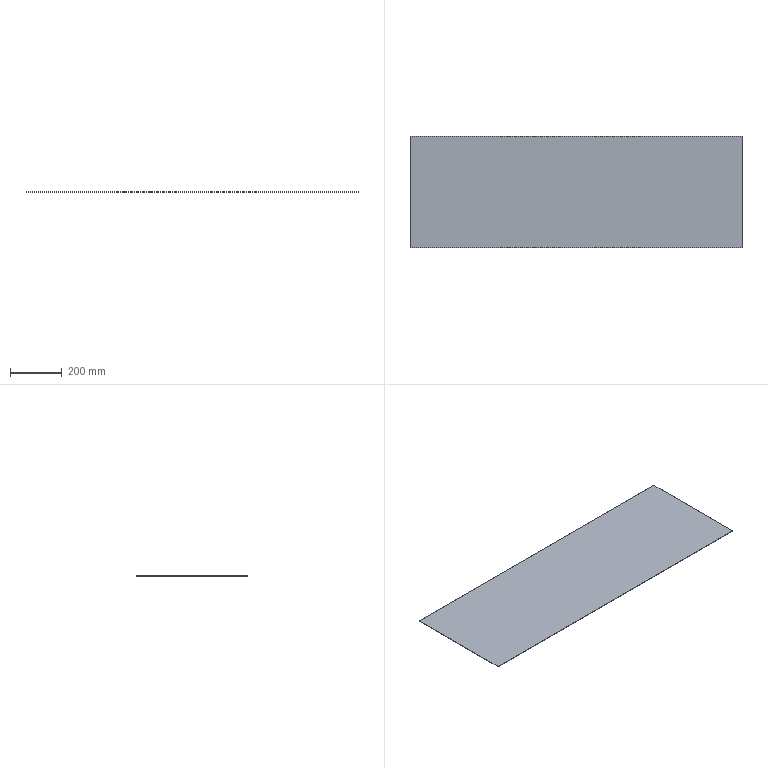Part | SolidWorks | features Extrusion 1 | 1 solid | 6 faces | box 1280 x 430 x 1.5 mm | volume 825600 mm3 | plane 6
STEP:
#1=CARTESIAN_POINT('',(0.,430.,0.));
#2=VERTEX_POINT('',#1);
#3=CARTESIAN_POINT('',(0.,0.,0.));
#4=VERTEX_POINT('',#3);
#5=CARTESIAN_POINT('',(0.,0.,0.));
#6=DIRECTION('',(0.,-1.,0.));
#7=VECTOR('',#6,1000.);
#8=LINE('',#5,#7);
#9=EDGE_CURVE('',#2,#4,#8,.T.);
#10=ORIENTED_EDGE('',*,*,#9,.T.);
#11=CARTESIAN_POINT('',(0.,0.,1.5));
#12=VERTEX_POINT('',#11);
#13=CARTESIAN_POINT('',(0.,0.,1.5));
#14=DIRECTION('',(0.,0.,-1.));
#15=VECTOR('',#14,1000.);
#16=LINE('',#13,#15);
#17=EDGE_CURVE('',#12,#4,#16,.T.);
#18=ORIENTED_EDGE('',*,*,#17,.F.);
#19=CARTESIAN_POINT('',(0.,430.,1.5));
#20=VERTEX_POINT('',#19);
#21=CARTESIAN_POINT('',(0.,0.,1.5));
#22=DIRECTION('',(0.,-1.,0.));
#23=VECTOR('',#22,1000.);
#24=LINE('',#21,#23);
#25=EDGE_CURVE('',#20,#12,#24,.T.);
#26=ORIENTED_EDGE('',*,*,#25,.F.);
#27=CARTESIAN_POINT('',(0.,430.,1.5));
#28=DIRECTION('',(0.,0.,-1.));
#29=VECTOR('',#28,1000.);
#30=LINE('',#27,#29);
#31=EDGE_CURVE('',#20,#2,#30,.T.);
#32=ORIENTED_EDGE('',*,*,#31,.T.);
#33=EDGE_LOOP('',(#10,#18,#26,#32));
#34=FACE_OUTER_BOUND('',#33,.T.);
#35=CARTESIAN_POINT('',(0.,0.,1.5));
#36=DIRECTION('',(1.,0.,0.));
#37=DIRECTION('',(0.,0.,-1.));
#38=AXIS2_PLACEMENT_3D('',#35,#36,#37);
#39=PLANE('',#38);
#40=ADVANCED_FACE('',(#34),#39,.F.);
#41=CARTESIAN_POINT('',(1280.,0.,0.));
#42=VERTEX_POINT('',#41);
#43=CARTESIAN_POINT('',(0.,0.,0.));
#44=DIRECTION('',(1.,0.,0.));
#45=VECTOR('',#44,1000.);
#46=LINE('',#43,#45);
#47=EDGE_CURVE('',#4,#42,#46,.T.);
#48=ORIENTED_EDGE('',*,*,#47,.T.);
#49=CARTESIAN_POINT('',(1280.,0.,1.5));
#50=VERTEX_POINT('',#49);
#51=CARTESIAN_POINT('',(1280.,0.,1.5));
#52=DIRECTION('',(0.,0.,-1.));
#53=VECTOR('',#52,1000.);
#54=LINE('',#51,#53);
#55=EDGE_CURVE('',#50,#42,#54,.T.);
#56=ORIENTED_EDGE('',*,*,#55,.F.);
#57=CARTESIAN_POINT('',(0.,0.,1.5));
#58=DIRECTION('',(1.,0.,0.));
#59=VECTOR('',#58,1000.);
#60=LINE('',#57,#59);
#61=EDGE_CURVE('',#12,#50,#60,.T.);
#62=ORIENTED_EDGE('',*,*,#61,.F.);
#63=ORIENTED_EDGE('',*,*,#17,.T.);
#64=EDGE_LOOP('',(#48,#56,#62,#63));
#65=FACE_OUTER_BOUND('',#64,.T.);
#66=CARTESIAN_POINT('',(0.,0.,1.5));
#67=DIRECTION('',(0.,1.,0.));
#68=DIRECTION('',(0.,0.,1.));
#69=AXIS2_PLACEMENT_3D('',#66,#67,#68);
#70=PLANE('',#69);
#71=ADVANCED_FACE('',(#65),#70,.F.);
#72=CARTESIAN_POINT('',(1280.,430.,0.));
#73=VERTEX_POINT('',#72);
#74=CARTESIAN_POINT('',(1280.,0.,0.));
#75=DIRECTION('',(0.,1.,0.));
#76=VECTOR('',#75,1000.);
#77=LINE('',#74,#76);
#78=EDGE_CURVE('',#42,#73,#77,.T.);
#79=ORIENTED_EDGE('',*,*,#78,.T.);
#80=CARTESIAN_POINT('',(1280.,430.,1.5));
#81=VERTEX_POINT('',#80);
#82=CARTESIAN_POINT('',(1280.,430.,1.5));
#83=DIRECTION('',(0.,0.,-1.));
#84=VECTOR('',#83,1000.);
#85=LINE('',#82,#84);
#86=EDGE_CURVE('',#81,#73,#85,.T.);
#87=ORIENTED_EDGE('',*,*,#86,.F.);
#88=CARTESIAN_POINT('',(1280.,0.,1.5));
#89=DIRECTION('',(0.,1.,0.));
#90=VECTOR('',#89,1000.);
#91=LINE('',#88,#90);
#92=EDGE_CURVE('',#50,#81,#91,.T.);
#93=ORIENTED_EDGE('',*,*,#92,.F.);
#94=ORIENTED_EDGE('',*,*,#55,.T.);
#95=EDGE_LOOP('',(#79,#87,#93,#94));
#96=FACE_OUTER_BOUND('',#95,.T.);
#97=CARTESIAN_POINT('',(1280.,0.,1.5));
#98=DIRECTION('',(-1.,0.,0.));
#99=DIRECTION('',(0.,0.,1.));
#100=AXIS2_PLACEMENT_3D('',#97,#98,#99);
#101=PLANE('',#100);
#102=ADVANCED_FACE('',(#96),#101,.F.);
#103=CARTESIAN_POINT('',(0.,430.,0.));
#104=DIRECTION('',(-1.,0.,0.));
#105=VECTOR('',#104,1000.);
#106=LINE('',#103,#105);
#107=EDGE_CURVE('',#73,#2,#106,.T.);
#108=ORIENTED_EDGE('',*,*,#107,.T.);
#109=ORIENTED_EDGE('',*,*,#31,.F.);
#110=CARTESIAN_POINT('',(0.,430.,1.5));
#111=DIRECTION('',(-1.,0.,0.));
#112=VECTOR('',#111,1000.);
#113=LINE('',#110,#112);
#114=EDGE_CURVE('',#81,#20,#113,.T.);
#115=ORIENTED_EDGE('',*,*,#114,.F.);
#116=ORIENTED_EDGE('',*,*,#86,.T.);
#117=EDGE_LOOP('',(#108,#109,#115,#116));
#118=FACE_OUTER_BOUND('',#117,.T.);
#119=CARTESIAN_POINT('',(0.,430.,1.5));
#120=DIRECTION('',(0.,-1.,0.));
#121=DIRECTION('',(0.,0.,-1.));
#122=AXIS2_PLACEMENT_3D('',#119,#120,#121);
#123=PLANE('',#122);
#124=ADVANCED_FACE('',(#118),#123,.F.);
#125=ORIENTED_EDGE('',*,*,#25,.T.);
#126=ORIENTED_EDGE('',*,*,#61,.T.);
#127=ORIENTED_EDGE('',*,*,#92,.T.);
#128=ORIENTED_EDGE('',*,*,#114,.T.);
#129=EDGE_LOOP('',(#125,#126,#127,#128));
#130=FACE_OUTER_BOUND('',#129,.T.);
#131=CARTESIAN_POINT('',(0.,0.,1.5));
#132=DIRECTION('',(0.,0.,-1.));
#133=DIRECTION('',(-1.,0.,0.));
#134=AXIS2_PLACEMENT_3D('',#131,#132,#133);
#135=PLANE('',#134);
#136=ADVANCED_FACE('',(#130),#135,.F.);
#137=ORIENTED_EDGE('',*,*,#9,.F.);
#138=ORIENTED_EDGE('',*,*,#107,.F.);
#139=ORIENTED_EDGE('',*,*,#78,.F.);
#140=ORIENTED_EDGE('',*,*,#47,.F.);
#141=EDGE_LOOP('',(#137,#138,#139,#140));
#142=FACE_OUTER_BOUND('',#141,.T.);
#143=CARTESIAN_POINT('',(0.,0.,0.));
#144=DIRECTION('',(0.,0.,-1.));
#145=DIRECTION('',(-1.,0.,0.));
#146=AXIS2_PLACEMENT_3D('',#143,#144,#145);
#147=PLANE('',#146);
#148=ADVANCED_FACE('',(#142),#147,.T.);
#149=CLOSED_SHELL('',(#40,#71,#102,#124,#136,#148));
#150=MANIFOLD_SOLID_BREP('',#149);
#151=CARTESIAN_POINT('',(0.,0.,0.));
#152=DIRECTION('',(0.,0.,1.));
#153=DIRECTION('',(1.,0.,0.));
#154=AXIS2_PLACEMENT_3D('',#151,#152,#153);
#155=(LENGTH_UNIT()NAMED_UNIT(*)SI_UNIT(.MILLI.,.METRE.));
#156=UNCERTAINTY_MEASURE_WITH_UNIT(LENGTH_MEASURE(0.00001),#155,'','');
#157=(NAMED_UNIT(*)PLANE_ANGLE_UNIT()SI_UNIT($,.RADIAN.));
#158=(NAMED_UNIT(*)SI_UNIT($,.STERADIAN.)SOLID_ANGLE_UNIT());
#159=(GEOMETRIC_REPRESENTATION_CONTEXT(3)GLOBAL_UNCERTAINTY_ASSIGNED_CONTEXT((#156))GLOBAL_UNIT_ASSIGNED_CONTEXT((#155,#157,#158))REPRESENTATION_CONTEXT('',''));
#160=ADVANCED_BREP_SHAPE_REPRESENTATION('',(#150,#154),#159);